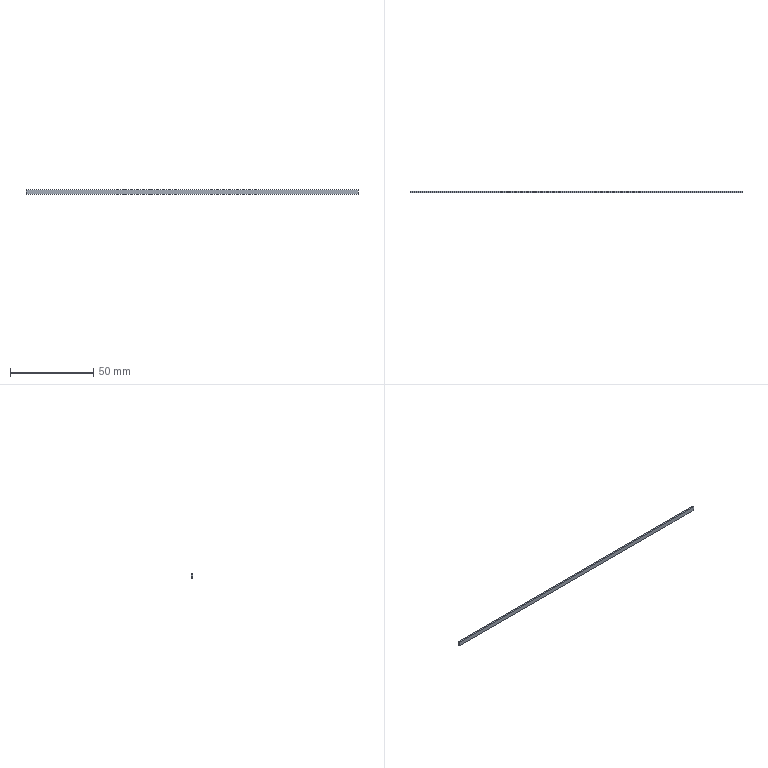Part | STEP file | TKR26H40-HS200 | 1 solid | 6 faces | box 200 x 1 x 2.6 mm | volume 520 mm3 | plane 6
STEP:
#1=CARTESIAN_POINT('',(0.,0.,0.));
#2=DIRECTION('',(0.,0.,1.));
#3=DIRECTION('',(1.,0.,0.));
#4=AXIS2_PLACEMENT_3D('',#1,#2,#3);
#5=CARTESIAN_POINT('',(0.,40.,0.));
#6=VERTEX_POINT('',#5);
#7=CARTESIAN_POINT('',(0.,39.,0.));
#8=VERTEX_POINT('',#7);
#9=CARTESIAN_POINT('',(0.,39.5,0.));
#10=DIRECTION('',(0.,-1.,0.));
#11=VECTOR('',#10,1.);
#12=LINE('',#9,#11);
#13=CARTESIAN_POINT('',(100.,39.5,0.));
#14=DIRECTION('',(0.,0.,-1.));
#15=DIRECTION('',(0.,1.,0.));
#16=AXIS2_PLACEMENT_3D('',#13,#14,#15);
#17=PLANE('',#16);
#18=CARTESIAN_POINT('',(0.,-100.));
#19=DIRECTION('',(-1.,0.));
#20=VECTOR('',#19,1.);
#21=LINE('',#18,#20);
#22=(GEOMETRIC_REPRESENTATION_CONTEXT(2)PARAMETRIC_REPRESENTATION_CONTEXT()REPRESENTATION_CONTEXT('',''));
#23=DEFINITIONAL_REPRESENTATION('',(#21),#22);
#24=PCURVE('',#17,#23);
#25=CARTESIAN_POINT('',(0.,39.5,2.6));
#26=DIRECTION('',(-1.,0.,0.));
#27=DIRECTION('',(0.,0.,1.));
#28=AXIS2_PLACEMENT_3D('',#25,#26,#27);
#29=PLANE('',#28);
#30=CARTESIAN_POINT('',(-2.6,0.));
#31=DIRECTION('',(0.,-1.));
#32=VECTOR('',#31,1.);
#33=LINE('',#30,#32);
#34=(GEOMETRIC_REPRESENTATION_CONTEXT(2)PARAMETRIC_REPRESENTATION_CONTEXT()REPRESENTATION_CONTEXT('',''));
#35=DEFINITIONAL_REPRESENTATION('',(#33),#34);
#36=PCURVE('',#29,#35);
#37=SURFACE_CURVE('',#12,(#24,#36),.PCURVE_S1.);
#38=EDGE_CURVE('',#6,#8,#37,.T.);
#39=ORIENTED_EDGE('',*,*,#38,.F.);
#40=CARTESIAN_POINT('',(200.,40.,0.));
#41=VERTEX_POINT('',#40);
#42=CARTESIAN_POINT('',(100.,40.,0.));
#43=DIRECTION('',(-1.,0.,0.));
#44=VECTOR('',#43,1.);
#45=LINE('',#42,#44);
#46=CARTESIAN_POINT('',(0.5,0.));
#47=DIRECTION('',(0.,-1.));
#48=VECTOR('',#47,1.);
#49=LINE('',#46,#48);
#50=(GEOMETRIC_REPRESENTATION_CONTEXT(2)PARAMETRIC_REPRESENTATION_CONTEXT()REPRESENTATION_CONTEXT('',''));
#51=DEFINITIONAL_REPRESENTATION('',(#49),#50);
#52=PCURVE('',#17,#51);
#53=CARTESIAN_POINT('',(100.,40.,2.6));
#54=DIRECTION('',(0.,1.,0.));
#55=DIRECTION('',(0.,0.,1.));
#56=AXIS2_PLACEMENT_3D('',#53,#54,#55);
#57=PLANE('',#56);
#58=CARTESIAN_POINT('',(-2.6,0.));
#59=DIRECTION('',(0.,-1.));
#60=VECTOR('',#59,1.);
#61=LINE('',#58,#60);
#62=(GEOMETRIC_REPRESENTATION_CONTEXT(2)PARAMETRIC_REPRESENTATION_CONTEXT()REPRESENTATION_CONTEXT('',''));
#63=DEFINITIONAL_REPRESENTATION('',(#61),#62);
#64=PCURVE('',#57,#63);
#65=SURFACE_CURVE('',#45,(#52,#64),.PCURVE_S1.);
#66=EDGE_CURVE('',#41,#6,#65,.T.);
#67=ORIENTED_EDGE('',*,*,#66,.F.);
#68=CARTESIAN_POINT('',(200.,39.,0.));
#69=VERTEX_POINT('',#68);
#70=CARTESIAN_POINT('',(200.,39.5,0.));
#71=DIRECTION('',(0.,1.,0.));
#72=VECTOR('',#71,1.);
#73=LINE('',#70,#72);
#74=CARTESIAN_POINT('',(0.,100.));
#75=DIRECTION('',(1.,0.));
#76=VECTOR('',#75,1.);
#77=LINE('',#74,#76);
#78=(GEOMETRIC_REPRESENTATION_CONTEXT(2)PARAMETRIC_REPRESENTATION_CONTEXT()REPRESENTATION_CONTEXT('',''));
#79=DEFINITIONAL_REPRESENTATION('',(#77),#78);
#80=PCURVE('',#17,#79);
#81=CARTESIAN_POINT('',(200.,39.5,2.6));
#82=DIRECTION('',(1.,0.,0.));
#83=DIRECTION('',(0.,0.,-1.));
#84=AXIS2_PLACEMENT_3D('',#81,#82,#83);
#85=PLANE('',#84);
#86=CARTESIAN_POINT('',(2.6,0.));
#87=DIRECTION('',(0.,1.));
#88=VECTOR('',#87,1.);
#89=LINE('',#86,#88);
#90=(GEOMETRIC_REPRESENTATION_CONTEXT(2)PARAMETRIC_REPRESENTATION_CONTEXT()REPRESENTATION_CONTEXT('',''));
#91=DEFINITIONAL_REPRESENTATION('',(#89),#90);
#92=PCURVE('',#85,#91);
#93=SURFACE_CURVE('',#73,(#80,#92),.PCURVE_S1.);
#94=EDGE_CURVE('',#69,#41,#93,.T.);
#95=ORIENTED_EDGE('',*,*,#94,.F.);
#96=CARTESIAN_POINT('',(100.,39.,0.));
#97=DIRECTION('',(1.,0.,0.));
#98=VECTOR('',#97,1.);
#99=LINE('',#96,#98);
#100=CARTESIAN_POINT('',(-0.5,0.));
#101=DIRECTION('',(0.,1.));
#102=VECTOR('',#101,1.);
#103=LINE('',#100,#102);
#104=(GEOMETRIC_REPRESENTATION_CONTEXT(2)PARAMETRIC_REPRESENTATION_CONTEXT()REPRESENTATION_CONTEXT('',''));
#105=DEFINITIONAL_REPRESENTATION('',(#103),#104);
#106=PCURVE('',#17,#105);
#107=CARTESIAN_POINT('',(100.,39.,2.6));
#108=DIRECTION('',(0.,-1.,0.));
#109=DIRECTION('',(0.,0.,-1.));
#110=AXIS2_PLACEMENT_3D('',#107,#108,#109);
#111=PLANE('',#110);
#112=CARTESIAN_POINT('',(2.6,0.));
#113=DIRECTION('',(0.,1.));
#114=VECTOR('',#113,1.);
#115=LINE('',#112,#114);
#116=(GEOMETRIC_REPRESENTATION_CONTEXT(2)PARAMETRIC_REPRESENTATION_CONTEXT()REPRESENTATION_CONTEXT('',''));
#117=DEFINITIONAL_REPRESENTATION('',(#115),#116);
#118=PCURVE('',#111,#117);
#119=SURFACE_CURVE('',#99,(#106,#118),.PCURVE_S1.);
#120=EDGE_CURVE('',#8,#69,#119,.T.);
#121=ORIENTED_EDGE('',*,*,#120,.F.);
#122=EDGE_LOOP('',(#39,#67,#95,#121));
#123=FACE_BOUND('',#122,.T.);
#124=ADVANCED_FACE('',(#123),#17,.T.);
#125=CARTESIAN_POINT('',(0.,40.,2.6));
#126=VERTEX_POINT('',#125);
#127=CARTESIAN_POINT('',(0.,40.,2.6));
#128=DIRECTION('',(0.,0.,-1.));
#129=VECTOR('',#128,1.);
#130=LINE('',#127,#129);
#131=CARTESIAN_POINT('',(0.,0.5));
#132=DIRECTION('',(-1.,0.));
#133=VECTOR('',#132,1.);
#134=LINE('',#131,#133);
#135=(GEOMETRIC_REPRESENTATION_CONTEXT(2)PARAMETRIC_REPRESENTATION_CONTEXT()REPRESENTATION_CONTEXT('',''));
#136=DEFINITIONAL_REPRESENTATION('',(#134),#135);
#137=PCURVE('',#29,#136);
#138=CARTESIAN_POINT('',(0.,-100.));
#139=DIRECTION('',(-1.,0.));
#140=VECTOR('',#139,1.);
#141=LINE('',#138,#140);
#142=(GEOMETRIC_REPRESENTATION_CONTEXT(2)PARAMETRIC_REPRESENTATION_CONTEXT()REPRESENTATION_CONTEXT('',''));
#143=DEFINITIONAL_REPRESENTATION('',(#141),#142);
#144=PCURVE('',#57,#143);
#145=SURFACE_CURVE('',#130,(#137,#144),.PCURVE_S1.);
#146=EDGE_CURVE('',#126,#6,#145,.T.);
#147=ORIENTED_EDGE('',*,*,#146,.T.);
#148=ORIENTED_EDGE('',*,*,#38,.T.);
#149=CARTESIAN_POINT('',(0.,39.,2.6));
#150=VERTEX_POINT('',#149);
#151=CARTESIAN_POINT('',(0.,39.,2.6));
#152=DIRECTION('',(0.,0.,-1.));
#153=VECTOR('',#152,1.);
#154=LINE('',#151,#153);
#155=CARTESIAN_POINT('',(0.,-0.5));
#156=DIRECTION('',(-1.,0.));
#157=VECTOR('',#156,1.);
#158=LINE('',#155,#157);
#159=(GEOMETRIC_REPRESENTATION_CONTEXT(2)PARAMETRIC_REPRESENTATION_CONTEXT()REPRESENTATION_CONTEXT('',''));
#160=DEFINITIONAL_REPRESENTATION('',(#158),#159);
#161=PCURVE('',#29,#160);
#162=CARTESIAN_POINT('',(0.,-100.));
#163=DIRECTION('',(1.,0.));
#164=VECTOR('',#163,1.);
#165=LINE('',#162,#164);
#166=(GEOMETRIC_REPRESENTATION_CONTEXT(2)PARAMETRIC_REPRESENTATION_CONTEXT()REPRESENTATION_CONTEXT('',''));
#167=DEFINITIONAL_REPRESENTATION('',(#165),#166);
#168=PCURVE('',#111,#167);
#169=SURFACE_CURVE('',#154,(#161,#168),.PCURVE_S1.);
#170=EDGE_CURVE('',#150,#8,#169,.T.);
#171=ORIENTED_EDGE('',*,*,#170,.F.);
#172=CARTESIAN_POINT('',(0.,39.5,2.6));
#173=DIRECTION('',(0.,1.,0.));
#174=VECTOR('',#173,1.);
#175=LINE('',#172,#174);
#176=CARTESIAN_POINT('',(0.,0.));
#177=DIRECTION('',(0.,1.));
#178=VECTOR('',#177,1.);
#179=LINE('',#176,#178);
#180=(GEOMETRIC_REPRESENTATION_CONTEXT(2)PARAMETRIC_REPRESENTATION_CONTEXT()REPRESENTATION_CONTEXT('',''));
#181=DEFINITIONAL_REPRESENTATION('',(#179),#180);
#182=PCURVE('',#29,#181);
#183=CARTESIAN_POINT('',(100.,39.5,2.6));
#184=DIRECTION('',(0.,0.,1.));
#185=DIRECTION('',(0.,-1.,0.));
#186=AXIS2_PLACEMENT_3D('',#183,#184,#185);
#187=PLANE('',#186);
#188=CARTESIAN_POINT('',(0.,-100.));
#189=DIRECTION('',(-1.,0.));
#190=VECTOR('',#189,1.);
#191=LINE('',#188,#190);
#192=(GEOMETRIC_REPRESENTATION_CONTEXT(2)PARAMETRIC_REPRESENTATION_CONTEXT()REPRESENTATION_CONTEXT('',''));
#193=DEFINITIONAL_REPRESENTATION('',(#191),#192);
#194=PCURVE('',#187,#193);
#195=SURFACE_CURVE('',#175,(#182,#194),.PCURVE_S1.);
#196=EDGE_CURVE('',#150,#126,#195,.T.);
#197=ORIENTED_EDGE('',*,*,#196,.T.);
#198=EDGE_LOOP('',(#147,#148,#171,#197));
#199=FACE_BOUND('',#198,.T.);
#200=ADVANCED_FACE('',(#199),#29,.T.);
#201=ORIENTED_EDGE('',*,*,#170,.T.);
#202=ORIENTED_EDGE('',*,*,#120,.T.);
#203=CARTESIAN_POINT('',(200.,39.,2.6));
#204=VERTEX_POINT('',#203);
#205=CARTESIAN_POINT('',(200.,39.,2.6));
#206=DIRECTION('',(0.,0.,-1.));
#207=VECTOR('',#206,1.);
#208=LINE('',#205,#207);
#209=CARTESIAN_POINT('',(0.,100.));
#210=DIRECTION('',(1.,0.));
#211=VECTOR('',#210,1.);
#212=LINE('',#209,#211);
#213=(GEOMETRIC_REPRESENTATION_CONTEXT(2)PARAMETRIC_REPRESENTATION_CONTEXT()REPRESENTATION_CONTEXT('',''));
#214=DEFINITIONAL_REPRESENTATION('',(#212),#213);
#215=PCURVE('',#111,#214);
#216=CARTESIAN_POINT('',(0.,-0.5));
#217=DIRECTION('',(1.,0.));
#218=VECTOR('',#217,1.);
#219=LINE('',#216,#218);
#220=(GEOMETRIC_REPRESENTATION_CONTEXT(2)PARAMETRIC_REPRESENTATION_CONTEXT()REPRESENTATION_CONTEXT('',''));
#221=DEFINITIONAL_REPRESENTATION('',(#219),#220);
#222=PCURVE('',#85,#221);
#223=SURFACE_CURVE('',#208,(#215,#222),.PCURVE_S1.);
#224=EDGE_CURVE('',#204,#69,#223,.T.);
#225=ORIENTED_EDGE('',*,*,#224,.F.);
#226=CARTESIAN_POINT('',(100.,39.,2.6));
#227=DIRECTION('',(-1.,0.,0.));
#228=VECTOR('',#227,1.);
#229=LINE('',#226,#228);
#230=CARTESIAN_POINT('',(0.,0.));
#231=DIRECTION('',(0.,-1.));
#232=VECTOR('',#231,1.);
#233=LINE('',#230,#232);
#234=(GEOMETRIC_REPRESENTATION_CONTEXT(2)PARAMETRIC_REPRESENTATION_CONTEXT()REPRESENTATION_CONTEXT('',''));
#235=DEFINITIONAL_REPRESENTATION('',(#233),#234);
#236=PCURVE('',#111,#235);
#237=CARTESIAN_POINT('',(0.5,0.));
#238=DIRECTION('',(0.,-1.));
#239=VECTOR('',#238,1.);
#240=LINE('',#237,#239);
#241=(GEOMETRIC_REPRESENTATION_CONTEXT(2)PARAMETRIC_REPRESENTATION_CONTEXT()REPRESENTATION_CONTEXT('',''));
#242=DEFINITIONAL_REPRESENTATION('',(#240),#241);
#243=PCURVE('',#187,#242);
#244=SURFACE_CURVE('',#229,(#236,#243),.PCURVE_S1.);
#245=EDGE_CURVE('',#204,#150,#244,.T.);
#246=ORIENTED_EDGE('',*,*,#245,.T.);
#247=EDGE_LOOP('',(#201,#202,#225,#246));
#248=FACE_BOUND('',#247,.T.);
#249=ADVANCED_FACE('',(#248),#111,.T.);
#250=ORIENTED_EDGE('',*,*,#224,.T.);
#251=ORIENTED_EDGE('',*,*,#94,.T.);
#252=CARTESIAN_POINT('',(200.,40.,2.6));
#253=VERTEX_POINT('',#252);
#254=CARTESIAN_POINT('',(200.,40.,2.6));
#255=DIRECTION('',(0.,0.,-1.));
#256=VECTOR('',#255,1.);
#257=LINE('',#254,#256);
#258=CARTESIAN_POINT('',(0.,0.5));
#259=DIRECTION('',(1.,0.));
#260=VECTOR('',#259,1.);
#261=LINE('',#258,#260);
#262=(GEOMETRIC_REPRESENTATION_CONTEXT(2)PARAMETRIC_REPRESENTATION_CONTEXT()REPRESENTATION_CONTEXT('',''));
#263=DEFINITIONAL_REPRESENTATION('',(#261),#262);
#264=PCURVE('',#85,#263);
#265=CARTESIAN_POINT('',(0.,100.));
#266=DIRECTION('',(-1.,0.));
#267=VECTOR('',#266,1.);
#268=LINE('',#265,#267);
#269=(GEOMETRIC_REPRESENTATION_CONTEXT(2)PARAMETRIC_REPRESENTATION_CONTEXT()REPRESENTATION_CONTEXT('',''));
#270=DEFINITIONAL_REPRESENTATION('',(#268),#269);
#271=PCURVE('',#57,#270);
#272=SURFACE_CURVE('',#257,(#264,#271),.PCURVE_S1.);
#273=EDGE_CURVE('',#253,#41,#272,.T.);
#274=ORIENTED_EDGE('',*,*,#273,.F.);
#275=CARTESIAN_POINT('',(200.,39.5,2.6));
#276=DIRECTION('',(0.,-1.,0.));
#277=VECTOR('',#276,1.);
#278=LINE('',#275,#277);
#279=CARTESIAN_POINT('',(0.,0.));
#280=DIRECTION('',(0.,-1.));
#281=VECTOR('',#280,1.);
#282=LINE('',#279,#281);
#283=(GEOMETRIC_REPRESENTATION_CONTEXT(2)PARAMETRIC_REPRESENTATION_CONTEXT()REPRESENTATION_CONTEXT('',''));
#284=DEFINITIONAL_REPRESENTATION('',(#282),#283);
#285=PCURVE('',#85,#284);
#286=CARTESIAN_POINT('',(0.,100.));
#287=DIRECTION('',(1.,0.));
#288=VECTOR('',#287,1.);
#289=LINE('',#286,#288);
#290=(GEOMETRIC_REPRESENTATION_CONTEXT(2)PARAMETRIC_REPRESENTATION_CONTEXT()REPRESENTATION_CONTEXT('',''));
#291=DEFINITIONAL_REPRESENTATION('',(#289),#290);
#292=PCURVE('',#187,#291);
#293=SURFACE_CURVE('',#278,(#285,#292),.PCURVE_S1.);
#294=EDGE_CURVE('',#253,#204,#293,.T.);
#295=ORIENTED_EDGE('',*,*,#294,.T.);
#296=EDGE_LOOP('',(#250,#251,#274,#295));
#297=FACE_BOUND('',#296,.T.);
#298=ADVANCED_FACE('',(#297),#85,.T.);
#299=CARTESIAN_POINT('',(100.,40.,2.6));
#300=DIRECTION('',(1.,0.,0.));
#301=VECTOR('',#300,1.);
#302=LINE('',#299,#301);
#303=CARTESIAN_POINT('',(-0.5,0.));
#304=DIRECTION('',(0.,1.));
#305=VECTOR('',#304,1.);
#306=LINE('',#303,#305);
#307=(GEOMETRIC_REPRESENTATION_CONTEXT(2)PARAMETRIC_REPRESENTATION_CONTEXT()REPRESENTATION_CONTEXT('',''));
#308=DEFINITIONAL_REPRESENTATION('',(#306),#307);
#309=PCURVE('',#187,#308);
#310=CARTESIAN_POINT('',(0.,0.));
#311=DIRECTION('',(0.,1.));
#312=VECTOR('',#311,1.);
#313=LINE('',#310,#312);
#314=(GEOMETRIC_REPRESENTATION_CONTEXT(2)PARAMETRIC_REPRESENTATION_CONTEXT()REPRESENTATION_CONTEXT('',''));
#315=DEFINITIONAL_REPRESENTATION('',(#313),#314);
#316=PCURVE('',#57,#315);
#317=SURFACE_CURVE('',#302,(#309,#316),.PCURVE_S1.);
#318=EDGE_CURVE('',#126,#253,#317,.T.);
#319=ORIENTED_EDGE('',*,*,#318,.F.);
#320=ORIENTED_EDGE('',*,*,#196,.F.);
#321=ORIENTED_EDGE('',*,*,#245,.F.);
#322=ORIENTED_EDGE('',*,*,#294,.F.);
#323=EDGE_LOOP('',(#319,#320,#321,#322));
#324=FACE_BOUND('',#323,.T.);
#325=ADVANCED_FACE('',(#324),#187,.T.);
#326=ORIENTED_EDGE('',*,*,#318,.T.);
#327=ORIENTED_EDGE('',*,*,#273,.T.);
#328=ORIENTED_EDGE('',*,*,#66,.T.);
#329=ORIENTED_EDGE('',*,*,#146,.F.);
#330=EDGE_LOOP('',(#326,#327,#328,#329));
#331=FACE_BOUND('',#330,.T.);
#332=ADVANCED_FACE('',(#331),#57,.T.);
#333=CLOSED_SHELL('',(#124,#200,#249,#298,#325,#332));
#334=MANIFOLD_SOLID_BREP('',#333);
#335=(LENGTH_UNIT()NAMED_UNIT(*)SI_UNIT(.MILLI.,.METRE.));
#336=UNCERTAINTY_MEASURE_WITH_UNIT(LENGTH_MEASURE(0.0000001),#335,'','');
#337=(NAMED_UNIT(*)PLANE_ANGLE_UNIT()SI_UNIT($,.RADIAN.));
#338=(NAMED_UNIT(*)SI_UNIT($,.STERADIAN.)SOLID_ANGLE_UNIT());
#339=(GEOMETRIC_REPRESENTATION_CONTEXT(3)GLOBAL_UNCERTAINTY_ASSIGNED_CONTEXT((#336))GLOBAL_UNIT_ASSIGNED_CONTEXT((#335,#337,#338))REPRESENTATION_CONTEXT('',''));
#340=ADVANCED_BREP_SHAPE_REPRESENTATION('',(#4,#334),#339);